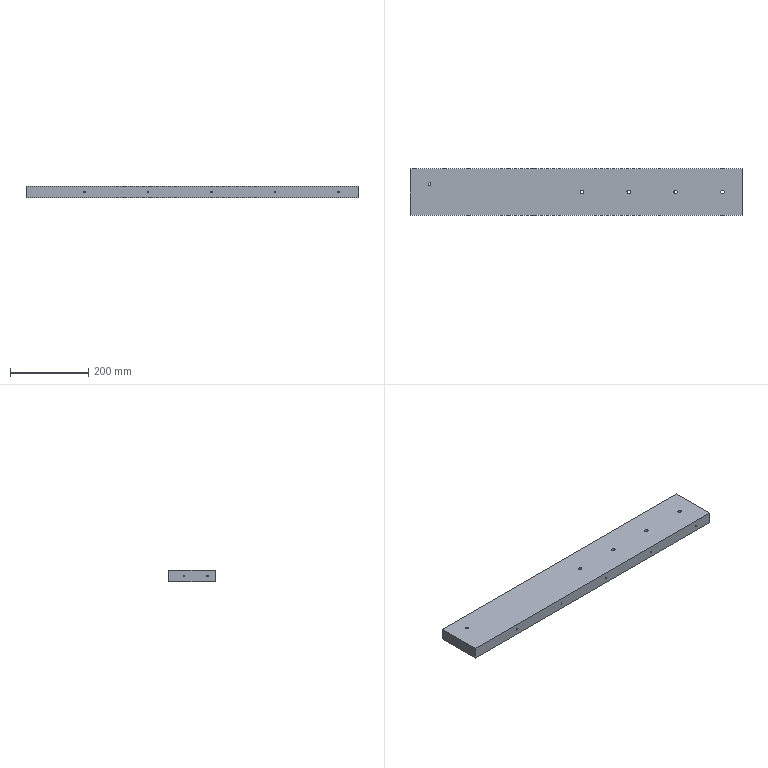CAM job | NX | 3-axis milling, drilling | part box 850 x 120 x 30 mm | stock box 855 x 125 x 30 mm
Tools:
number,name,description,diameter,corner_radius,flute_length,length,flutes
4,D4,平底铣刀-粗,4.0,0.0,25.0,75.0,2
9,D10,平底铣刀-粗,10.0,0.0,35.0,75.0,2
10,D10-J,平底铣刀-精,10.0,0.0,35.0,75.0,2
2,D6倒角刀,倒角刀,6.0,0.0,3.0,25.0,2
17,ZT9,钻头,9.0,0.0,35.0,50.0,2
16,ZT6.9,Drilling Tool,6.9,0.0,35.0,50.0,2
Operations:
program,operation,operation_type,tool,method,geometry_group,spindle_rpm,surface_speed,feed_per_tooth,feed_cut,feed_plunge,cut_length_mm,path_length_mm,cut_time_min,machine_time_min
A,打点-深0.8,Operation,D6倒角刀,NONE,W-A,8000.0,150.796,0.0312,500.0,90.0,9.0,872.526,0.018,0.1044
A,通孔-M8螺纹底孔,Operation,ZT6.9,NONE,W-A,1800.0,38.453,0.0972,350.0,90.0,30.5,161.0,0.0871,0.1002
A,通孔-8-10,Operation,ZT9,NONE,W-A,1800.0,50.894,0.0417,150.0,90.0,122.0,707.013,0.8133,0.8718
A,底壁铣螺旋精光-中_COPY,VolumeBased25DMillingOperation,D4,螺旋精光-切深K-步距G,W-A,8000.0,100.531,0.0312,500.0,100.0,4427.713,5819.976,8.855,8.995
A,外形粗_2,VolumeBased25DMillingOperation,D10,METHOD,W-A,6000.0,188.0,0.25,4000.0,80.0,120296.202,120424.202,30.074,30.087
A,仅选体,SurfaceContour,D6倒角刀,METHOD,W-A,6000.0,113.0,0.125,1200.0,100.0,1957.315,2053.116,1.631,1.641
A,铣倒角_3,PlanarMilling,D6倒角刀,METHOD,W-A,8000.0,150.796,0.0312,500.0,100.0,24.401,126.001,0.0488,0.059
A,铣倒角_4,PlanarMilling,D6倒角刀,METHOD,W-A,8000.0,150.796,0.0375,600.0,100.0,139.642,904.008,0.2327,0.3092
A,外形半精_2,VolumeBased25DMillingOperation,D10-J,METHOD,W-A,6000.0,113.0,0.0833,1000.0,100.0,5929.122,6349.151,5.929,5.971
A,外形精_2,VolumeBased25DMillingOperation,D10-J,METHOD,W-A,6000.0,113.0,0.0833,1000.0,100.0,1976.174,2134.774,1.976,1.992